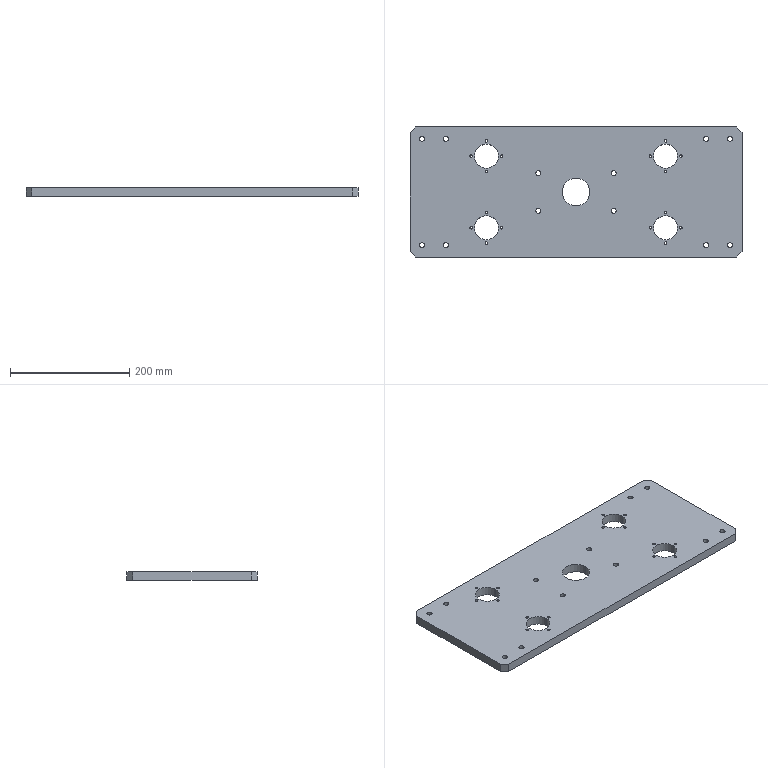Part | SolidWorks | features BaseBody 1 | 1 solid | 100 faces | box 556 x 218 x 15 mm | volume 1694256 mm3 | cylinder 82 | plane 18 | commonest cylinder face diameters 4.2 x32 8.5 x24 14 x16 40 x8 46 x2